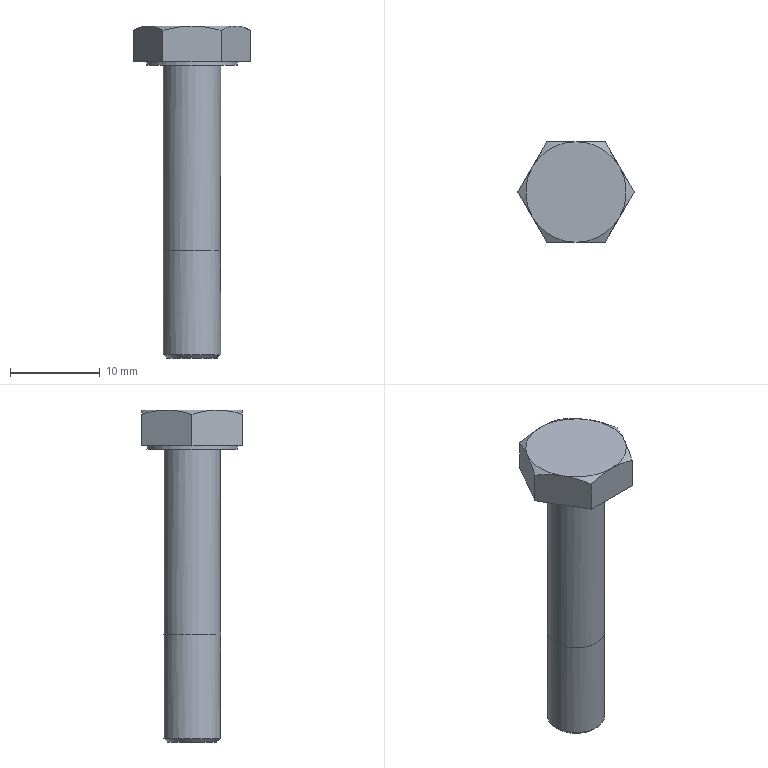Part | NX | features solid 2 | 1 solid | 20 faces | box 12.905 x 11.176 x 36.913 mm | volume 1489 mm3 | plane 10 | cone 7 | cylinder 3 | commonest cylinder face diameters 6.35 x2 10.109 x1
STEP:
#1=CARTESIAN_POINT('',(-3.175,0.,-4.369));
#2=VERTEX_POINT('',#1);
#3=CARTESIAN_POINT('',(0.,0.,-4.369));
#4=DIRECTION('',(0.,0.,-1.));
#5=DIRECTION('',(-1.,0.,0.));
#6=AXIS2_PLACEMENT_3D('',#3,#4,#5);
#7=CIRCLE('',#6,3.175);
#8=EDGE_CURVE('',#2,#2,#7,.T.);
#9=ORIENTED_EDGE('',*,*,#8,.T.);
#10=EDGE_LOOP('',(#9));
#11=FACE_BOUND('',#10,.T.);
#12=CARTESIAN_POINT('',(-3.175,0.,-25.006));
#13=VERTEX_POINT('',#12);
#14=CARTESIAN_POINT('',(-2.488,2.488,-25.006));
#15=CARTESIAN_POINT('',(-3.519,0.,-25.006));
#16=CARTESIAN_POINT('',(-2.488,-2.488,-25.006));
#17=CARTESIAN_POINT('',(0.,-3.519,-25.006));
#18=CARTESIAN_POINT('',(2.488,-2.488,-25.006));
#19=CARTESIAN_POINT('',(3.519,0.,-25.006));
#20=CARTESIAN_POINT('',(2.488,2.488,-25.006));
#21=CARTESIAN_POINT('',(0.,3.519,-25.006));
#22=CARTESIAN_POINT('',(-2.488,2.488,-25.006));
#23=CARTESIAN_POINT('',(-3.519,0.,-25.006));
#24=CARTESIAN_POINT('',(-2.488,-2.488,-25.006));
#25=B_SPLINE_CURVE_WITH_KNOTS('',3,(#14,#15,#16,#17,#18,#19,#20,#21,#22,#23,#24),.UNSPECIFIED.,.T.,.F.,(1,1,1,1,1,1,1,1,1,1,1,1,1,1,1),(-0.375,-0.25,-0.125,0.,0.125,0.25,0.375,0.5,0.625,0.75,0.875,1.,1.125,1.25,1.375),.UNSPECIFIED.);
#26=EDGE_CURVE('',#13,#13,#25,.T.);
#27=ORIENTED_EDGE('',*,*,#26,.T.);
#28=EDGE_LOOP('',(#27));
#29=FACE_BOUND('',#28,.T.);
#30=CARTESIAN_POINT('',(0.,0.,0.));
#31=DIRECTION('',(0.,0.,-1.));
#32=DIRECTION('',(-1.,0.,0.));
#33=AXIS2_PLACEMENT_3D('',#30,#31,#32);
#34=CYLINDRICAL_SURFACE('',#33,3.175);
#35=ADVANCED_FACE('',(#11,#29),#34,.T.);
#36=CARTESIAN_POINT('',(-6.452,0.,-3.962));
#37=VERTEX_POINT('',#36);
#38=CARTESIAN_POINT('',(-3.226,5.588,-3.962));
#39=VERTEX_POINT('',#38);
#40=CARTESIAN_POINT('',(-3.576,4.983,-3.962));
#41=DIRECTION('',(0.5,0.866,0.));
#42=VECTOR('',#41,1000.);
#43=LINE('',#40,#42);
#44=EDGE_CURVE('',#37,#39,#43,.T.);
#45=ORIENTED_EDGE('',*,*,#44,.T.);
#46=CARTESIAN_POINT('',(3.226,5.588,-3.962));
#47=VERTEX_POINT('',#46);
#48=CARTESIAN_POINT('',(5.055,5.588,-3.962));
#49=DIRECTION('',(1.,0.,0.));
#50=VECTOR('',#49,1000.);
#51=LINE('',#48,#50);
#52=EDGE_CURVE('',#39,#47,#51,.T.);
#53=ORIENTED_EDGE('',*,*,#52,.T.);
#54=CARTESIAN_POINT('',(6.452,0.,-3.962));
#55=VERTEX_POINT('',#54);
#56=CARTESIAN_POINT('',(6.103,0.6053,-3.962));
#57=DIRECTION('',(0.5,-0.866,0.));
#58=VECTOR('',#57,1000.);
#59=LINE('',#56,#58);
#60=EDGE_CURVE('',#47,#55,#59,.T.);
#61=ORIENTED_EDGE('',*,*,#60,.T.);
#62=CARTESIAN_POINT('',(3.226,-5.588,-3.962));
#63=VERTEX_POINT('',#62);
#64=CARTESIAN_POINT('',(6.103,-0.6053,-3.962));
#65=DIRECTION('',(-0.5,-0.866,0.));
#66=VECTOR('',#65,1000.);
#67=LINE('',#64,#66);
#68=EDGE_CURVE('',#55,#63,#67,.T.);
#69=ORIENTED_EDGE('',*,*,#68,.T.);
#70=CARTESIAN_POINT('',(-3.226,-5.588,-3.962));
#71=VERTEX_POINT('',#70);
#72=CARTESIAN_POINT('',(5.055,-5.588,-3.962));
#73=DIRECTION('',(-1.,0.,0.));
#74=VECTOR('',#73,1000.);
#75=LINE('',#72,#74);
#76=EDGE_CURVE('',#63,#71,#75,.T.);
#77=ORIENTED_EDGE('',*,*,#76,.T.);
#78=CARTESIAN_POINT('',(-3.576,-4.983,-3.962));
#79=DIRECTION('',(-0.5,0.866,0.));
#80=VECTOR('',#79,1000.);
#81=LINE('',#78,#80);
#82=EDGE_CURVE('',#71,#37,#81,.T.);
#83=ORIENTED_EDGE('',*,*,#82,.T.);
#84=EDGE_LOOP('',(#45,#53,#61,#69,#77,#83));
#85=FACE_BOUND('',#84,.T.);
#86=CARTESIAN_POINT('',(-5.055,0.,-3.962));
#87=VERTEX_POINT('',#86);
#88=CARTESIAN_POINT('',(0.,0.,-3.962));
#89=DIRECTION('',(0.,0.,-1.));
#90=DIRECTION('',(-1.,0.,0.));
#91=AXIS2_PLACEMENT_3D('',#88,#89,#90);
#92=CIRCLE('',#91,5.055);
#93=EDGE_CURVE('',#87,#87,#92,.T.);
#94=ORIENTED_EDGE('',*,*,#93,.F.);
#95=EDGE_LOOP('',(#94));
#96=FACE_BOUND('',#95,.T.);
#97=CARTESIAN_POINT('',(5.055,0.,-3.962));
#98=DIRECTION('',(0.,0.,-1.));
#99=DIRECTION('',(-1.,0.,0.));
#100=AXIS2_PLACEMENT_3D('',#97,#98,#99);
#101=PLANE('',#100);
#102=ADVANCED_FACE('',(#85,#96),#101,.T.);
#103=CARTESIAN_POINT('',(-2.794,0.,-36.913));
#104=VERTEX_POINT('',#103);
#105=CARTESIAN_POINT('',(0.,0.,-36.913));
#106=DIRECTION('',(0.,0.,-1.));
#107=DIRECTION('',(-1.,0.,0.));
#108=AXIS2_PLACEMENT_3D('',#105,#106,#107);
#109=CIRCLE('',#108,2.794);
#110=EDGE_CURVE('',#104,#104,#109,.T.);
#111=ORIENTED_EDGE('',*,*,#110,.T.);
#112=EDGE_LOOP('',(#111));
#113=FACE_BOUND('',#112,.T.);
#114=CARTESIAN_POINT('',(0.,0.,-36.913));
#115=DIRECTION('',(0.,0.,-1.));
#116=DIRECTION('',(-1.,0.,0.));
#117=AXIS2_PLACEMENT_3D('',#114,#115,#116);
#118=PLANE('',#117);
#119=ADVANCED_FACE('',(#113),#118,.T.);
#120=CARTESIAN_POINT('',(-3.175,0.,-36.532));
#121=VERTEX_POINT('',#120);
#122=CARTESIAN_POINT('',(0.,0.,-36.532));
#123=DIRECTION('',(0.,0.,-1.));
#124=DIRECTION('',(-1.,0.,0.));
#125=AXIS2_PLACEMENT_3D('',#122,#123,#124);
#126=CIRCLE('',#125,3.175);
#127=EDGE_CURVE('',#121,#121,#126,.T.);
#128=ORIENTED_EDGE('',*,*,#127,.T.);
#129=EDGE_LOOP('',(#128));
#130=FACE_BOUND('',#129,.T.);
#131=ORIENTED_EDGE('',*,*,#110,.F.);
#132=EDGE_LOOP('',(#131));
#133=FACE_BOUND('',#132,.T.);
#134=CARTESIAN_POINT('',(0.,0.,-36.913));
#135=DIRECTION('',(0.,0.,1.));
#136=DIRECTION('',(1.,0.,0.));
#137=AXIS2_PLACEMENT_3D('',#134,#135,#136);
#138=CONICAL_SURFACE('',#137,2.794,0.7854);
#139=ADVANCED_FACE('',(#130,#133),#138,.T.);
#140=ORIENTED_EDGE('',*,*,#26,.F.);
#141=EDGE_LOOP('',(#140));
#142=FACE_BOUND('',#141,.T.);
#143=ORIENTED_EDGE('',*,*,#127,.F.);
#144=EDGE_LOOP('',(#143));
#145=FACE_BOUND('',#144,.T.);
#146=CARTESIAN_POINT('',(0.,0.,0.));
#147=DIRECTION('',(0.,0.,-1.));
#148=DIRECTION('',(-1.,0.,0.));
#149=AXIS2_PLACEMENT_3D('',#146,#147,#148);
#150=CYLINDRICAL_SURFACE('',#149,3.175);
#151=ADVANCED_FACE('',(#142,#145),#150,.T.);
#152=CARTESIAN_POINT('',(-5.055,0.,-4.369));
#153=VERTEX_POINT('',#152);
#154=CARTESIAN_POINT('',(0.,0.,-4.369));
#155=DIRECTION('',(0.,0.,-1.));
#156=DIRECTION('',(-1.,0.,0.));
#157=AXIS2_PLACEMENT_3D('',#154,#155,#156);
#158=CIRCLE('',#157,5.055);
#159=EDGE_CURVE('',#153,#153,#158,.T.);
#160=ORIENTED_EDGE('',*,*,#159,.T.);
#161=EDGE_LOOP('',(#160));
#162=FACE_BOUND('',#161,.T.);
#163=ORIENTED_EDGE('',*,*,#8,.F.);
#164=EDGE_LOOP('',(#163));
#165=FACE_BOUND('',#164,.T.);
#166=CARTESIAN_POINT('',(3.175,0.,-4.369));
#167=DIRECTION('',(0.,0.,-1.));
#168=DIRECTION('',(-1.,0.,0.));
#169=AXIS2_PLACEMENT_3D('',#166,#167,#168);
#170=PLANE('',#169);
#171=ADVANCED_FACE('',(#162,#165),#170,.T.);
#172=ORIENTED_EDGE('',*,*,#93,.T.);
#173=EDGE_LOOP('',(#172));
#174=FACE_BOUND('',#173,.T.);
#175=ORIENTED_EDGE('',*,*,#159,.F.);
#176=EDGE_LOOP('',(#175));
#177=FACE_BOUND('',#176,.T.);
#178=CARTESIAN_POINT('',(0.,0.,0.));
#179=DIRECTION('',(0.,0.,-1.));
#180=DIRECTION('',(-1.,0.,0.));
#181=AXIS2_PLACEMENT_3D('',#178,#179,#180);
#182=CYLINDRICAL_SURFACE('',#181,5.055);
#183=ADVANCED_FACE('',(#174,#177),#182,.T.);
#184=ORIENTED_EDGE('',*,*,#52,.F.);
#185=CARTESIAN_POINT('',(-3.226,5.588,-0.4991));
#186=VERTEX_POINT('',#185);
#187=CARTESIAN_POINT('',(-3.226,5.588,-40.604));
#188=DIRECTION('',(0.,0.,1.));
#189=VECTOR('',#188,1000.);
#190=LINE('',#187,#189);
#191=EDGE_CURVE('',#39,#186,#190,.T.);
#192=ORIENTED_EDGE('',*,*,#191,.T.);
#193=CARTESIAN_POINT('',(0.,5.588,0.));
#194=VERTEX_POINT('',#193);
#195=CARTESIAN_POINT('',(-3.226,5.588,-0.4991));
#196=CARTESIAN_POINT('',(-2.177,5.588,-0.1961));
#197=CARTESIAN_POINT('',(-1.09,5.588,0.));
#198=CARTESIAN_POINT('',(0.,5.588,0.));
#199=B_SPLINE_CURVE_WITH_KNOTS('',3,(#195,#196,#197,#198),.UNSPECIFIED.,.F.,.F.,(4,4),(0.005758,0.009022),.UNSPECIFIED.);
#200=EDGE_CURVE('',#194,#186,#199,.F.);
#201=ORIENTED_EDGE('',*,*,#200,.F.);
#202=CARTESIAN_POINT('',(3.226,5.588,-0.4991));
#203=VERTEX_POINT('',#202);
#204=CARTESIAN_POINT('',(0.,5.588,0.));
#205=CARTESIAN_POINT('',(1.091,5.588,0.));
#206=CARTESIAN_POINT('',(2.183,5.588,-0.1979));
#207=CARTESIAN_POINT('',(3.226,5.588,-0.4991));
#208=B_SPLINE_CURVE_WITH_KNOTS('',3,(#204,#205,#206,#207),.UNSPECIFIED.,.F.,.F.,(4,4),(0.009022,0.01229),.UNSPECIFIED.);
#209=EDGE_CURVE('',#203,#194,#208,.F.);
#210=ORIENTED_EDGE('',*,*,#209,.F.);
#211=CARTESIAN_POINT('',(3.226,5.588,-40.604));
#212=DIRECTION('',(0.,0.,1.));
#213=VECTOR('',#212,1000.);
#214=LINE('',#211,#213);
#215=EDGE_CURVE('',#47,#203,#214,.T.);
#216=ORIENTED_EDGE('',*,*,#215,.F.);
#217=EDGE_LOOP('',(#184,#192,#201,#210,#216));
#218=FACE_BOUND('',#217,.T.);
#219=CARTESIAN_POINT('',(3.226,5.588,-40.604));
#220=DIRECTION('',(0.,1.,0.));
#221=DIRECTION('',(0.,0.,1.));
#222=AXIS2_PLACEMENT_3D('',#219,#220,#221);
#223=PLANE('',#222);
#224=ADVANCED_FACE('',(#218),#223,.T.);
#225=ORIENTED_EDGE('',*,*,#44,.F.);
#226=CARTESIAN_POINT('',(-6.452,0.,-0.4991));
#227=VERTEX_POINT('',#226);
#228=CARTESIAN_POINT('',(-6.452,0.,-40.604));
#229=DIRECTION('',(0.,0.,1.));
#230=VECTOR('',#229,1000.);
#231=LINE('',#228,#230);
#232=EDGE_CURVE('',#37,#227,#231,.T.);
#233=ORIENTED_EDGE('',*,*,#232,.T.);
#234=CARTESIAN_POINT('',(-4.839,2.794,0.));
#235=VERTEX_POINT('',#234);
#236=CARTESIAN_POINT('',(-4.839,2.794,0.));
#237=CARTESIAN_POINT('',(-5.387,1.846,0.));
#238=CARTESIAN_POINT('',(-5.926,0.9118,-0.1952));
#239=CARTESIAN_POINT('',(-6.452,0.,-0.4991));
#240=B_SPLINE_CURVE_WITH_KNOTS('',3,(#236,#237,#238,#239),.UNSPECIFIED.,.F.,.F.,(4,4),(0.003265,0.006517),.UNSPECIFIED.);
#241=EDGE_CURVE('',#235,#227,#240,.T.);
#242=ORIENTED_EDGE('',*,*,#241,.F.);
#243=CARTESIAN_POINT('',(-3.226,5.588,-0.4991));
#244=CARTESIAN_POINT('',(-3.754,4.674,-0.1944));
#245=CARTESIAN_POINT('',(-4.29,3.746,0.));
#246=CARTESIAN_POINT('',(-4.839,2.794,0.));
#247=B_SPLINE_CURVE_WITH_KNOTS('',3,(#243,#244,#245,#246),.UNSPECIFIED.,.F.,.F.,(4,4),(0.000000238,0.003265),.UNSPECIFIED.);
#248=EDGE_CURVE('',#186,#235,#247,.T.);
#249=ORIENTED_EDGE('',*,*,#248,.F.);
#250=ORIENTED_EDGE('',*,*,#191,.F.);
#251=EDGE_LOOP('',(#225,#233,#242,#249,#250));
#252=FACE_BOUND('',#251,.T.);
#253=CARTESIAN_POINT('',(-3.226,5.588,-40.604));
#254=DIRECTION('',(-0.866,0.5,0.));
#255=DIRECTION('',(-0.5,-0.866,0.));
#256=AXIS2_PLACEMENT_3D('',#253,#254,#255);
#257=PLANE('',#256);
#258=ADVANCED_FACE('',(#252),#257,.T.);
#259=ORIENTED_EDGE('',*,*,#82,.F.);
#260=CARTESIAN_POINT('',(-3.226,-5.588,-0.4991));
#261=VERTEX_POINT('',#260);
#262=CARTESIAN_POINT('',(-3.226,-5.588,-40.604));
#263=DIRECTION('',(0.,0.,1.));
#264=VECTOR('',#263,1000.);
#265=LINE('',#262,#264);
#266=EDGE_CURVE('',#71,#261,#265,.T.);
#267=ORIENTED_EDGE('',*,*,#266,.T.);
#268=CARTESIAN_POINT('',(-4.839,-2.794,0.));
#269=VERTEX_POINT('',#268);
#270=CARTESIAN_POINT('',(-4.839,-2.794,0.));
#271=CARTESIAN_POINT('',(-4.292,-3.742,0.));
#272=CARTESIAN_POINT('',(-3.753,-4.676,-0.1952));
#273=CARTESIAN_POINT('',(-3.226,-5.588,-0.4991));
#274=B_SPLINE_CURVE_WITH_KNOTS('',3,(#270,#271,#272,#273),.UNSPECIFIED.,.F.,.F.,(4,4),(0.003265,0.006517),.UNSPECIFIED.);
#275=EDGE_CURVE('',#269,#261,#274,.T.);
#276=ORIENTED_EDGE('',*,*,#275,.F.);
#277=CARTESIAN_POINT('',(-6.452,0.,-0.4991));
#278=CARTESIAN_POINT('',(-5.925,-0.9141,-0.1944));
#279=CARTESIAN_POINT('',(-5.389,-1.842,0.));
#280=CARTESIAN_POINT('',(-4.839,-2.794,0.));
#281=B_SPLINE_CURVE_WITH_KNOTS('',3,(#277,#278,#279,#280),.UNSPECIFIED.,.F.,.F.,(4,4),(0.000000238,0.003265),.UNSPECIFIED.);
#282=EDGE_CURVE('',#227,#269,#281,.T.);
#283=ORIENTED_EDGE('',*,*,#282,.F.);
#284=ORIENTED_EDGE('',*,*,#232,.F.);
#285=EDGE_LOOP('',(#259,#267,#276,#283,#284));
#286=FACE_BOUND('',#285,.T.);
#287=CARTESIAN_POINT('',(-6.452,0.,-40.604));
#288=DIRECTION('',(-0.866,-0.5,0.));
#289=DIRECTION('',(0.5,-0.866,0.));
#290=AXIS2_PLACEMENT_3D('',#287,#288,#289);
#291=PLANE('',#290);
#292=ADVANCED_FACE('',(#286),#291,.T.);
#293=ORIENTED_EDGE('',*,*,#76,.F.);
#294=CARTESIAN_POINT('',(3.226,-5.588,-0.4991));
#295=VERTEX_POINT('',#294);
#296=CARTESIAN_POINT('',(3.226,-5.588,-40.604));
#297=DIRECTION('',(0.,0.,1.));
#298=VECTOR('',#297,1000.);
#299=LINE('',#296,#298);
#300=EDGE_CURVE('',#63,#295,#299,.T.);
#301=ORIENTED_EDGE('',*,*,#300,.T.);
#302=CARTESIAN_POINT('',(0.,-5.588,0.));
#303=VERTEX_POINT('',#302);
#304=CARTESIAN_POINT('',(0.,-5.588,0.));
#305=CARTESIAN_POINT('',(1.091,-5.588,0.));
#306=CARTESIAN_POINT('',(2.183,-5.588,-0.1979));
#307=CARTESIAN_POINT('',(3.226,-5.588,-0.4991));
#308=B_SPLINE_CURVE_WITH_KNOTS('',3,(#304,#305,#306,#307),.UNSPECIFIED.,.F.,.F.,(4,4),(0.009022,0.01229),.UNSPECIFIED.);
#309=EDGE_CURVE('',#303,#295,#308,.T.);
#310=ORIENTED_EDGE('',*,*,#309,.F.);
#311=CARTESIAN_POINT('',(-3.226,-5.588,-0.4991));
#312=CARTESIAN_POINT('',(-2.177,-5.588,-0.1961));
#313=CARTESIAN_POINT('',(-1.09,-5.588,0.));
#314=CARTESIAN_POINT('',(0.,-5.588,0.));
#315=B_SPLINE_CURVE_WITH_KNOTS('',3,(#311,#312,#313,#314),.UNSPECIFIED.,.F.,.F.,(4,4),(0.005758,0.009022),.UNSPECIFIED.);
#316=EDGE_CURVE('',#261,#303,#315,.T.);
#317=ORIENTED_EDGE('',*,*,#316,.F.);
#318=ORIENTED_EDGE('',*,*,#266,.F.);
#319=EDGE_LOOP('',(#293,#301,#310,#317,#318));
#320=FACE_BOUND('',#319,.T.);
#321=CARTESIAN_POINT('',(-3.226,-5.588,-40.604));
#322=DIRECTION('',(0.,-1.,0.));
#323=DIRECTION('',(0.,0.,-1.));
#324=AXIS2_PLACEMENT_3D('',#321,#322,#323);
#325=PLANE('',#324);
#326=ADVANCED_FACE('',(#320),#325,.T.);
#327=ORIENTED_EDGE('',*,*,#68,.F.);
#328=CARTESIAN_POINT('',(6.452,0.,-0.4991));
#329=VERTEX_POINT('',#328);
#330=CARTESIAN_POINT('',(6.452,0.,-40.604));
#331=DIRECTION('',(0.,0.,1.));
#332=VECTOR('',#331,1000.);
#333=LINE('',#330,#332);
#334=EDGE_CURVE('',#55,#329,#333,.T.);
#335=ORIENTED_EDGE('',*,*,#334,.T.);
#336=CARTESIAN_POINT('',(4.839,-2.794,0.));
#337=VERTEX_POINT('',#336);
#338=CARTESIAN_POINT('',(4.839,-2.794,0.));
#339=CARTESIAN_POINT('',(5.387,-1.846,0.));
#340=CARTESIAN_POINT('',(5.926,-0.9118,-0.1952));
#341=CARTESIAN_POINT('',(6.452,0.,-0.4991));
#342=B_SPLINE_CURVE_WITH_KNOTS('',3,(#338,#339,#340,#341),.UNSPECIFIED.,.F.,.F.,(4,4),(0.003265,0.006517),.UNSPECIFIED.);
#343=EDGE_CURVE('',#337,#329,#342,.T.);
#344=ORIENTED_EDGE('',*,*,#343,.F.);
#345=CARTESIAN_POINT('',(3.226,-5.588,-0.4991));
#346=CARTESIAN_POINT('',(3.754,-4.674,-0.1944));
#347=CARTESIAN_POINT('',(4.29,-3.746,0.));
#348=CARTESIAN_POINT('',(4.839,-2.794,0.));
#349=B_SPLINE_CURVE_WITH_KNOTS('',3,(#345,#346,#347,#348),.UNSPECIFIED.,.F.,.F.,(4,4),(0.000000238,0.003265),.UNSPECIFIED.);
#350=EDGE_CURVE('',#295,#337,#349,.T.);
#351=ORIENTED_EDGE('',*,*,#350,.F.);
#352=ORIENTED_EDGE('',*,*,#300,.F.);
#353=EDGE_LOOP('',(#327,#335,#344,#351,#352));
#354=FACE_BOUND('',#353,.T.);
#355=CARTESIAN_POINT('',(3.226,-5.588,-40.604));
#356=DIRECTION('',(0.866,-0.5,0.));
#357=DIRECTION('',(0.5,0.866,0.));
#358=AXIS2_PLACEMENT_3D('',#355,#356,#357);
#359=PLANE('',#358);
#360=ADVANCED_FACE('',(#354),#359,.T.);
#361=ORIENTED_EDGE('',*,*,#60,.F.);
#362=ORIENTED_EDGE('',*,*,#215,.T.);
#363=CARTESIAN_POINT('',(4.839,2.794,0.));
#364=VERTEX_POINT('',#363);
#365=CARTESIAN_POINT('',(4.839,2.794,0.));
#366=CARTESIAN_POINT('',(4.292,3.742,0.));
#367=CARTESIAN_POINT('',(3.753,4.676,-0.1952));
#368=CARTESIAN_POINT('',(3.226,5.588,-0.4991));
#369=B_SPLINE_CURVE_WITH_KNOTS('',3,(#365,#366,#367,#368),.UNSPECIFIED.,.F.,.F.,(4,4),(0.003265,0.006517),.UNSPECIFIED.);
#370=EDGE_CURVE('',#364,#203,#369,.T.);
#371=ORIENTED_EDGE('',*,*,#370,.F.);
#372=CARTESIAN_POINT('',(6.452,0.,-0.4991));
#373=CARTESIAN_POINT('',(5.925,0.9141,-0.1944));
#374=CARTESIAN_POINT('',(5.389,1.842,0.));
#375=CARTESIAN_POINT('',(4.839,2.794,0.));
#376=B_SPLINE_CURVE_WITH_KNOTS('',3,(#372,#373,#374,#375),.UNSPECIFIED.,.F.,.F.,(4,4),(0.000000238,0.003265),.UNSPECIFIED.);
#377=EDGE_CURVE('',#329,#364,#376,.T.);
#378=ORIENTED_EDGE('',*,*,#377,.F.);
#379=ORIENTED_EDGE('',*,*,#334,.F.);
#380=EDGE_LOOP('',(#361,#362,#371,#378,#379));
#381=FACE_BOUND('',#380,.T.);
#382=CARTESIAN_POINT('',(6.452,0.,-40.604));
#383=DIRECTION('',(0.866,0.5,0.));
#384=DIRECTION('',(-0.5,0.866,0.));
#385=AXIS2_PLACEMENT_3D('',#382,#383,#384);
#386=PLANE('',#385);
#387=ADVANCED_FACE('',(#381),#386,.T.);
#388=CARTESIAN_POINT('',(0.,0.,0.));
#389=DIRECTION('',(0.,0.,-1.));
#390=DIRECTION('',(-1.,0.,0.));
#391=AXIS2_PLACEMENT_3D('',#388,#389,#390);
#392=CIRCLE('',#391,5.588);
#393=EDGE_CURVE('',#364,#337,#392,.T.);
#394=ORIENTED_EDGE('',*,*,#393,.T.);
#395=ORIENTED_EDGE('',*,*,#343,.T.);
#396=ORIENTED_EDGE('',*,*,#377,.T.);
#397=EDGE_LOOP('',(#394,#395,#396));
#398=FACE_BOUND('',#397,.T.);
#399=CARTESIAN_POINT('',(0.,0.,-0.5133));
#400=DIRECTION('',(0.,0.,-1.));
#401=DIRECTION('',(-1.,0.,0.));
#402=AXIS2_PLACEMENT_3D('',#399,#400,#401);
#403=CONICAL_SURFACE('',#402,6.477,1.047);
#404=ADVANCED_FACE('',(#398),#403,.T.);
#405=CARTESIAN_POINT('',(0.,0.,0.));
#406=DIRECTION('',(0.,0.,-1.));
#407=DIRECTION('',(-1.,0.,0.));
#408=AXIS2_PLACEMENT_3D('',#405,#406,#407);
#409=CIRCLE('',#408,5.588);
#410=EDGE_CURVE('',#337,#303,#409,.T.);
#411=ORIENTED_EDGE('',*,*,#410,.T.);
#412=ORIENTED_EDGE('',*,*,#309,.T.);
#413=ORIENTED_EDGE('',*,*,#350,.T.);
#414=EDGE_LOOP('',(#411,#412,#413));
#415=FACE_BOUND('',#414,.T.);
#416=CARTESIAN_POINT('',(0.,0.,-0.5133));
#417=DIRECTION('',(0.,0.,-1.));
#418=DIRECTION('',(-1.,0.,0.));
#419=AXIS2_PLACEMENT_3D('',#416,#417,#418);
#420=CONICAL_SURFACE('',#419,6.477,1.047);
#421=ADVANCED_FACE('',(#415),#420,.T.);
#422=CARTESIAN_POINT('',(0.,0.,0.));
#423=DIRECTION('',(0.,0.,-1.));
#424=DIRECTION('',(-1.,0.,0.));
#425=AXIS2_PLACEMENT_3D('',#422,#423,#424);
#426=CIRCLE('',#425,5.588);
#427=EDGE_CURVE('',#303,#269,#426,.T.);
#428=ORIENTED_EDGE('',*,*,#427,.T.);
#429=ORIENTED_EDGE('',*,*,#275,.T.);
#430=ORIENTED_EDGE('',*,*,#316,.T.);
#431=EDGE_LOOP('',(#428,#429,#430));
#432=FACE_BOUND('',#431,.T.);
#433=CARTESIAN_POINT('',(0.,0.,-0.5133));
#434=DIRECTION('',(0.,0.,-1.));
#435=DIRECTION('',(-1.,0.,0.));
#436=AXIS2_PLACEMENT_3D('',#433,#434,#435);
#437=CONICAL_SURFACE('',#436,6.477,1.047);
#438=ADVANCED_FACE('',(#432),#437,.T.);
#439=CARTESIAN_POINT('',(0.,0.,0.));
#440=DIRECTION('',(0.,0.,-1.));
#441=DIRECTION('',(-1.,0.,0.));
#442=AXIS2_PLACEMENT_3D('',#439,#440,#441);
#443=CIRCLE('',#442,5.588);
#444=EDGE_CURVE('',#269,#235,#443,.T.);
#445=ORIENTED_EDGE('',*,*,#444,.T.);
#446=ORIENTED_EDGE('',*,*,#241,.T.);
#447=ORIENTED_EDGE('',*,*,#282,.T.);
#448=EDGE_LOOP('',(#445,#446,#447));
#449=FACE_BOUND('',#448,.T.);
#450=CARTESIAN_POINT('',(0.,0.,-0.5133));
#451=DIRECTION('',(0.,0.,-1.));
#452=DIRECTION('',(-1.,0.,0.));
#453=AXIS2_PLACEMENT_3D('',#450,#451,#452);
#454=CONICAL_SURFACE('',#453,6.477,1.047);
#455=ADVANCED_FACE('',(#449),#454,.T.);
#456=CARTESIAN_POINT('',(0.,0.,0.));
#457=DIRECTION('',(0.,0.,-1.));
#458=DIRECTION('',(-1.,0.,0.));
#459=AXIS2_PLACEMENT_3D('',#456,#457,#458);
#460=CIRCLE('',#459,5.588);
#461=EDGE_CURVE('',#235,#194,#460,.T.);
#462=ORIENTED_EDGE('',*,*,#461,.T.);
#463=ORIENTED_EDGE('',*,*,#200,.T.);
#464=ORIENTED_EDGE('',*,*,#248,.T.);
#465=EDGE_LOOP('',(#462,#463,#464));
#466=FACE_BOUND('',#465,.T.);
#467=CARTESIAN_POINT('',(0.,0.,-0.5133));
#468=DIRECTION('',(0.,0.,-1.));
#469=DIRECTION('',(-1.,0.,0.));
#470=AXIS2_PLACEMENT_3D('',#467,#468,#469);
#471=CONICAL_SURFACE('',#470,6.477,1.047);
#472=ADVANCED_FACE('',(#466),#471,.T.);
#473=ORIENTED_EDGE('',*,*,#461,.F.);
#474=ORIENTED_EDGE('',*,*,#444,.F.);
#475=ORIENTED_EDGE('',*,*,#427,.F.);
#476=ORIENTED_EDGE('',*,*,#410,.F.);
#477=ORIENTED_EDGE('',*,*,#393,.F.);
#478=CARTESIAN_POINT('',(0.,0.,0.));
#479=DIRECTION('',(0.,0.,-1.));
#480=DIRECTION('',(-1.,0.,0.));
#481=AXIS2_PLACEMENT_3D('',#478,#479,#480);
#482=CIRCLE('',#481,5.588);
#483=EDGE_CURVE('',#194,#364,#482,.T.);
#484=ORIENTED_EDGE('',*,*,#483,.F.);
#485=EDGE_LOOP('',(#473,#474,#475,#476,#477,#484));
#486=FACE_BOUND('',#485,.T.);
#487=CARTESIAN_POINT('',(5.588,0.,0.));
#488=DIRECTION('',(0.,0.,1.));
#489=DIRECTION('',(1.,0.,0.));
#490=AXIS2_PLACEMENT_3D('',#487,#488,#489);
#491=PLANE('',#490);
#492=ADVANCED_FACE('',(#486),#491,.T.);
#493=ORIENTED_EDGE('',*,*,#370,.T.);
#494=ORIENTED_EDGE('',*,*,#209,.T.);
#495=ORIENTED_EDGE('',*,*,#483,.T.);
#496=EDGE_LOOP('',(#493,#494,#495));
#497=FACE_BOUND('',#496,.T.);
#498=CARTESIAN_POINT('',(0.,0.,-0.5133));
#499=DIRECTION('',(0.,0.,-1.));
#500=DIRECTION('',(-1.,0.,0.));
#501=AXIS2_PLACEMENT_3D('',#498,#499,#500);
#502=CONICAL_SURFACE('',#501,6.477,1.047);
#503=ADVANCED_FACE('',(#497),#502,.T.);
#504=CLOSED_SHELL('',(#35,#102,#119,#139,#151,#171,#183,#224,#258,#292,#326,#360,#387,#404,#421,#438,#455,#472,#492,#503));
#505=MANIFOLD_SOLID_BREP('',#504);
#506=(LENGTH_UNIT()NAMED_UNIT(*)SI_UNIT(.MILLI.,.METRE.));
#507=UNCERTAINTY_MEASURE_WITH_UNIT(LENGTH_MEASURE(0.0508),#506,'','');
#508=(NAMED_UNIT(*)PLANE_ANGLE_UNIT()SI_UNIT($,.RADIAN.));
#509=(NAMED_UNIT(*)SI_UNIT($,.STERADIAN.)SOLID_ANGLE_UNIT());
#510=(GEOMETRIC_REPRESENTATION_CONTEXT(3)GLOBAL_UNCERTAINTY_ASSIGNED_CONTEXT((#507))GLOBAL_UNIT_ASSIGNED_CONTEXT((#506,#508,#509))REPRESENTATION_CONTEXT('',''));
#511=ADVANCED_BREP_SHAPE_REPRESENTATION('',(#505),#510);